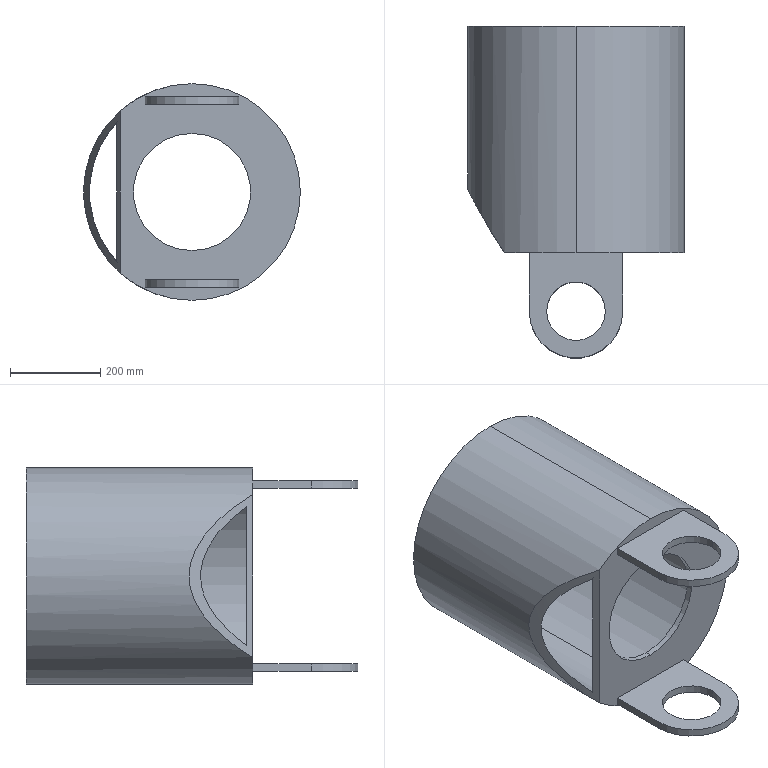Part | SolidWorks | features ICE 3, MoveFace 3, BaseBody 1, Scale 1 | 1 solid | 24 faces | box 481 x 737 x 481 mm | volume 11479821 mm3 | cylinder 13 | plane 11 | commonest cylinder face diameters 130 x4 208 x2 260 x2 455 x2 481 x2 2594 x1
STEP:
#1=CARTESIAN_POINT('',(65.,-174.262,211.9));
#2=VERTEX_POINT('',#1);
#3=CARTESIAN_POINT('',(-65.,-174.262,211.9));
#4=VERTEX_POINT('',#3);
#5=CARTESIAN_POINT('',(0.,-174.262,211.9));
#6=DIRECTION('',(0.,0.,-1.));
#7=DIRECTION('',(1.,0.,0.));
#8=AXIS2_PLACEMENT_3D('',#5,#6,#7);
#9=CIRCLE('',#8,65.);
#10=EDGE_CURVE('',#2,#4,#9,.T.);
#11=ORIENTED_EDGE('',*,*,#10,.F.);
#12=CARTESIAN_POINT('',(65.,-174.262,195.));
#13=VERTEX_POINT('',#12);
#14=CARTESIAN_POINT('',(65.,-174.262,428.84));
#15=DIRECTION('',(0.,0.,-1.));
#16=VECTOR('',#15,1000.);
#17=LINE('',#14,#16);
#18=EDGE_CURVE('',#2,#13,#17,.T.);
#19=ORIENTED_EDGE('',*,*,#18,.T.);
#20=CARTESIAN_POINT('',(-65.,-174.262,195.));
#21=VERTEX_POINT('',#20);
#22=CARTESIAN_POINT('',(0.,-174.262,195.));
#23=DIRECTION('',(0.,0.,-1.));
#24=DIRECTION('',(-1.,0.,0.));
#25=AXIS2_PLACEMENT_3D('',#22,#23,#24);
#26=CIRCLE('',#25,65.);
#27=EDGE_CURVE('',#13,#21,#26,.T.);
#28=ORIENTED_EDGE('',*,*,#27,.T.);
#29=CARTESIAN_POINT('',(-65.,-174.262,428.84));
#30=DIRECTION('',(0.,0.,-1.));
#31=VECTOR('',#30,1000.);
#32=LINE('',#29,#31);
#33=EDGE_CURVE('',#4,#21,#32,.T.);
#34=ORIENTED_EDGE('',*,*,#33,.F.);
#35=EDGE_LOOP('',(#11,#19,#28,#34));
#36=FACE_OUTER_BOUND('',#35,.T.);
#37=CARTESIAN_POINT('',(0.,-174.262,428.84));
#38=DIRECTION('',(0.,0.,-1.));
#39=DIRECTION('',(-1.,0.,0.));
#40=AXIS2_PLACEMENT_3D('',#37,#38,#39);
#41=CYLINDRICAL_SURFACE('',#40,65.);
#42=ADVANCED_FACE('',(#36),#41,.F.);
#43=CARTESIAN_POINT('',(-65.,-174.262,-195.));
#44=VERTEX_POINT('',#43);
#45=CARTESIAN_POINT('',(65.,-174.262,-195.));
#46=VERTEX_POINT('',#45);
#47=CARTESIAN_POINT('',(0.,-174.262,-195.));
#48=DIRECTION('',(0.,0.,1.));
#49=DIRECTION('',(-1.,0.,0.));
#50=AXIS2_PLACEMENT_3D('',#47,#48,#49);
#51=CIRCLE('',#50,65.);
#52=EDGE_CURVE('',#44,#46,#51,.T.);
#53=ORIENTED_EDGE('',*,*,#52,.T.);
#54=CARTESIAN_POINT('',(65.,-174.262,-211.9));
#55=VERTEX_POINT('',#54);
#56=CARTESIAN_POINT('',(65.,-174.262,21.94));
#57=DIRECTION('',(0.,0.,-1.));
#58=VECTOR('',#57,1000.);
#59=LINE('',#56,#58);
#60=EDGE_CURVE('',#46,#55,#59,.T.);
#61=ORIENTED_EDGE('',*,*,#60,.T.);
#62=CARTESIAN_POINT('',(-65.,-174.262,-211.9));
#63=VERTEX_POINT('',#62);
#64=CARTESIAN_POINT('',(0.,-174.262,-211.9));
#65=DIRECTION('',(0.,0.,-1.));
#66=DIRECTION('',(-1.,0.,0.));
#67=AXIS2_PLACEMENT_3D('',#64,#65,#66);
#68=CIRCLE('',#67,65.);
#69=EDGE_CURVE('',#55,#63,#68,.T.);
#70=ORIENTED_EDGE('',*,*,#69,.T.);
#71=CARTESIAN_POINT('',(-65.,-174.262,21.94));
#72=DIRECTION('',(0.,0.,-1.));
#73=VECTOR('',#72,1000.);
#74=LINE('',#71,#73);
#75=EDGE_CURVE('',#44,#63,#74,.T.);
#76=ORIENTED_EDGE('',*,*,#75,.F.);
#77=EDGE_LOOP('',(#53,#61,#70,#76));
#78=FACE_OUTER_BOUND('',#77,.T.);
#79=CARTESIAN_POINT('',(0.,-174.262,21.94));
#80=DIRECTION('',(0.,0.,-1.));
#81=DIRECTION('',(-1.,0.,0.));
#82=AXIS2_PLACEMENT_3D('',#79,#80,#81);
#83=CYLINDRICAL_SURFACE('',#82,65.);
#84=ADVANCED_FACE('',(#78),#83,.F.);
#85=CARTESIAN_POINT('',(0.,458.738,-240.5));
#86=VERTEX_POINT('',#85);
#87=CARTESIAN_POINT('',(0.,458.738,240.5));
#88=VERTEX_POINT('',#87);
#89=CARTESIAN_POINT('',(0.,458.738,0.));
#90=DIRECTION('',(0.,-1.,0.));
#91=DIRECTION('',(0.,0.,-1.));
#92=AXIS2_PLACEMENT_3D('',#89,#90,#91);
#93=CIRCLE('',#92,240.5);
#94=EDGE_CURVE('',#86,#88,#93,.T.);
#95=ORIENTED_EDGE('',*,*,#94,.T.);
#96=CARTESIAN_POINT('',(0.,-44.262,240.5));
#97=VERTEX_POINT('',#96);
#98=CARTESIAN_POINT('',(0.,358.738,240.5));
#99=DIRECTION('',(0.,-1.,0.));
#100=VECTOR('',#99,1000.);
#101=LINE('',#98,#100);
#102=EDGE_CURVE('',#88,#97,#101,.T.);
#103=ORIENTED_EDGE('',*,*,#102,.T.);
#104=CARTESIAN_POINT('',(0.,-44.262,-240.5));
#105=VERTEX_POINT('',#104);
#106=CARTESIAN_POINT('',(0.,-44.262,0.));
#107=DIRECTION('',(0.,1.,0.));
#108=DIRECTION('',(0.,0.,-1.));
#109=AXIS2_PLACEMENT_3D('',#106,#107,#108);
#110=CIRCLE('',#109,240.5);
#111=EDGE_CURVE('',#97,#105,#110,.T.);
#112=ORIENTED_EDGE('',*,*,#111,.T.);
#113=CARTESIAN_POINT('',(0.,358.738,-240.5));
#114=DIRECTION('',(0.,-1.,0.));
#115=VECTOR('',#114,1000.);
#116=LINE('',#113,#115);
#117=EDGE_CURVE('',#86,#105,#116,.T.);
#118=ORIENTED_EDGE('',*,*,#117,.F.);
#119=EDGE_LOOP('',(#95,#103,#112,#118));
#120=FACE_OUTER_BOUND('',#119,.T.);
#121=CARTESIAN_POINT('',(0.,358.738,0.));
#122=DIRECTION('',(0.,-1.,0.));
#123=DIRECTION('',(0.,0.,-1.));
#124=AXIS2_PLACEMENT_3D('',#121,#122,#123);
#125=CYLINDRICAL_SURFACE('',#124,240.5);
#126=ADVANCED_FACE('',(#120),#125,.T.);
#127=CARTESIAN_POINT('',(0.,-31.262,130.));
#128=VERTEX_POINT('',#127);
#129=CARTESIAN_POINT('',(0.,-31.262,-130.));
#130=VERTEX_POINT('',#129);
#131=CARTESIAN_POINT('',(0.,-31.262,0.));
#132=DIRECTION('',(0.,-1.,0.));
#133=DIRECTION('',(0.,0.,-1.));
#134=AXIS2_PLACEMENT_3D('',#131,#132,#133);
#135=CIRCLE('',#134,130.);
#136=EDGE_CURVE('',#128,#130,#135,.T.);
#137=ORIENTED_EDGE('',*,*,#136,.F.);
#138=CARTESIAN_POINT('',(0.,-44.262,130.));
#139=VERTEX_POINT('',#138);
#140=CARTESIAN_POINT('',(0.,358.738,130.));
#141=DIRECTION('',(0.,-1.,0.));
#142=VECTOR('',#141,1000.);
#143=LINE('',#140,#142);
#144=EDGE_CURVE('',#128,#139,#143,.T.);
#145=ORIENTED_EDGE('',*,*,#144,.T.);
#146=CARTESIAN_POINT('',(0.,-44.262,-130.));
#147=VERTEX_POINT('',#146);
#148=CARTESIAN_POINT('',(0.,-44.262,0.));
#149=DIRECTION('',(0.,1.,0.));
#150=DIRECTION('',(0.,0.,-1.));
#151=AXIS2_PLACEMENT_3D('',#148,#149,#150);
#152=CIRCLE('',#151,130.);
#153=EDGE_CURVE('',#147,#139,#152,.T.);
#154=ORIENTED_EDGE('',*,*,#153,.F.);
#155=CARTESIAN_POINT('',(0.,358.738,-130.));
#156=DIRECTION('',(0.,-1.,0.));
#157=VECTOR('',#156,1000.);
#158=LINE('',#155,#157);
#159=EDGE_CURVE('',#130,#147,#158,.T.);
#160=ORIENTED_EDGE('',*,*,#159,.F.);
#161=EDGE_LOOP('',(#137,#145,#154,#160));
#162=FACE_OUTER_BOUND('',#161,.T.);
#163=CARTESIAN_POINT('',(0.,358.738,0.));
#164=DIRECTION('',(0.,-1.,0.));
#165=DIRECTION('',(0.,0.,-1.));
#166=AXIS2_PLACEMENT_3D('',#163,#164,#165);
#167=CYLINDRICAL_SURFACE('',#166,130.);
#168=ADVANCED_FACE('',(#162),#167,.F.);
#169=CARTESIAN_POINT('',(0.,458.738,227.5));
#170=VERTEX_POINT('',#169);
#171=CARTESIAN_POINT('',(0.,458.738,-227.5));
#172=VERTEX_POINT('',#171);
#173=CARTESIAN_POINT('',(0.,458.738,0.));
#174=DIRECTION('',(0.,-1.,0.));
#175=DIRECTION('',(0.,0.,-1.));
#176=AXIS2_PLACEMENT_3D('',#173,#174,#175);
#177=CIRCLE('',#176,227.5);
#178=EDGE_CURVE('',#170,#172,#177,.T.);
#179=ORIENTED_EDGE('',*,*,#178,.F.);
#180=CARTESIAN_POINT('',(0.,-31.262,227.5));
#181=VERTEX_POINT('',#180);
#182=CARTESIAN_POINT('',(0.,358.738,227.5));
#183=DIRECTION('',(0.,-1.,0.));
#184=VECTOR('',#183,1000.);
#185=LINE('',#182,#184);
#186=EDGE_CURVE('',#170,#181,#185,.T.);
#187=ORIENTED_EDGE('',*,*,#186,.T.);
#188=CARTESIAN_POINT('',(-167.294,-31.262,154.171));
#189=VERTEX_POINT('',#188);
#190=CARTESIAN_POINT('',(0.,-31.262,0.));
#191=DIRECTION('',(0.,1.,0.));
#192=DIRECTION('',(0.,0.,-1.));
#193=AXIS2_PLACEMENT_3D('',#190,#191,#192);
#194=CIRCLE('',#193,227.5);
#195=EDGE_CURVE('',#189,#181,#194,.T.);
#196=ORIENTED_EDGE('',*,*,#195,.F.);
#197=CARTESIAN_POINT('',(-167.294,-31.262,-154.171));
#198=VERTEX_POINT('',#197);
#199=CARTESIAN_POINT('',(-167.294,-31.262,154.171));
#200=CARTESIAN_POINT('',(-171.27,-25.129,149.857));
#201=CARTESIAN_POINT('',(-175.109,-19.095,145.358));
#202=CARTESIAN_POINT('',(-182.509,-7.257,135.95));
#203=CARTESIAN_POINT('',(-186.07,-1.453,131.043));
#204=CARTESIAN_POINT('',(-192.904,9.87,120.758));
#205=CARTESIAN_POINT('',(-196.176,15.391,115.382));
#206=CARTESIAN_POINT('',(-202.406,26.071,104.066));
#207=CARTESIAN_POINT('',(-205.365,31.231,98.126));
#208=CARTESIAN_POINT('',(-209.534,38.606,88.677));
#209=CARTESIAN_POINT('',(-210.878,41.004,85.437));
#210=CARTESIAN_POINT('',(-212.82,44.491,80.418));
#211=CARTESIAN_POINT('',(-213.455,45.635,78.718));
#212=CARTESIAN_POINT('',(-214.689,47.867,75.287));
#213=CARTESIAN_POINT('',(-215.289,48.957,73.554));
#214=CARTESIAN_POINT('',(-217.039,52.143,68.294));
#215=CARTESIAN_POINT('',(-218.136,54.155,64.71));
#216=CARTESIAN_POINT('',(-220.181,57.927,57.367));
#217=CARTESIAN_POINT('',(-221.129,59.685,53.609));
#218=CARTESIAN_POINT('',(-222.426,62.104,47.821));
#219=CARTESIAN_POINT('',(-222.837,62.873,45.867));
#220=CARTESIAN_POINT('',(-223.422,63.968,42.896));
#221=CARTESIAN_POINT('',(-223.611,64.322,41.9));
#222=CARTESIAN_POINT('',(-223.975,65.007,39.905));
#223=CARTESIAN_POINT('',(-224.151,65.337,38.905));
#224=CARTESIAN_POINT('',(-224.998,66.932,33.889));
#225=CARTESIAN_POINT('',(-225.573,68.019,29.832));
#226=CARTESIAN_POINT('',(-226.508,69.789,21.62));
#227=CARTESIAN_POINT('',(-226.868,70.473,17.466));
#228=CARTESIAN_POINT('',(-227.236,71.174,11.158));
#229=CARTESIAN_POINT('',(-227.33,71.354,9.043));
#230=CARTESIAN_POINT('',(-227.427,71.538,5.849));
#231=CARTESIAN_POINT('',(-227.452,71.586,4.781));
#232=CARTESIAN_POINT('',(-227.487,71.653,2.639));
#233=CARTESIAN_POINT('',(-227.497,71.672,1.563));
#234=CARTESIAN_POINT('',(-227.518,71.711,-8.121));
#235=CARTESIAN_POINT('',(-227.05,70.816,-16.551));
#236=CARTESIAN_POINT('',(-225.915,68.666,-26.889));
#237=CARTESIAN_POINT('',(-225.66,68.184,-28.947));
#238=CARTESIAN_POINT('',(-225.097,67.119,-33.043));
#239=CARTESIAN_POINT('',(-224.788,66.536,-35.083));
#240=CARTESIAN_POINT('',(-223.782,64.643,-41.165));
#241=CARTESIAN_POINT('',(-223.018,63.208,-45.11));
#242=CARTESIAN_POINT('',(-221.321,60.042,-52.81));
#243=CARTESIAN_POINT('',(-220.389,58.311,-56.565));
#244=CARTESIAN_POINT('',(-218.373,54.59,-63.907));
#245=CARTESIAN_POINT('',(-217.289,52.6,-67.495));
#246=CARTESIAN_POINT('',(-215.557,49.444,-72.765));
#247=CARTESIAN_POINT('',(-214.962,48.363,-74.503));
#248=CARTESIAN_POINT('',(-213.739,46.148,-77.944));
#249=CARTESIAN_POINT('',(-213.109,45.012,-79.649));
#250=CARTESIAN_POINT('',(-211.18,41.544,-84.688));
#251=CARTESIAN_POINT('',(-209.842,39.154,-87.947));
#252=CARTESIAN_POINT('',(-205.683,31.788,-97.461));
#253=CARTESIAN_POINT('',(-202.72,26.615,-103.457));
#254=CARTESIAN_POINT('',(-196.461,15.874,-114.9));
#255=CARTESIAN_POINT('',(-193.163,10.305,-120.347));
#256=CARTESIAN_POINT('',(-187.985,1.717,-128.171));
#257=CARTESIAN_POINT('',(-186.22,-1.185,-130.721));
#258=CARTESIAN_POINT('',(-183.515,-5.592,-134.466));
#259=CARTESIAN_POINT('',(-182.603,-7.071,-135.701));
#260=CARTESIAN_POINT('',(-180.764,-10.041,-138.142));
#261=CARTESIAN_POINT('',(-179.836,-11.533,-139.347));
#262=CARTESIAN_POINT('',(-175.158,-19.019,-145.302));
#263=CARTESIAN_POINT('',(-171.288,-25.102,-149.838));
#264=CARTESIAN_POINT('',(-167.294,-31.262,-154.171));
#265=B_SPLINE_CURVE_WITH_KNOTS('',3,(#199,#200,#201,#202,#203,#204,#205,#206,#207,#208,#209,#210,#211,#212,#213,#214,#215,#216,#217,#218,#219,#220,#221,#222,#223,#224,#225,#226,#227,#228,#229,#230,#231,#232,#233,#234,#235,#236,#237,#238,#239,#240,#241,#242,#243,#244,#245,#246,#247,#248,#249,#250,#251,#252,#253,#254,#255,#256,#257,#258,#259,#260,#261,#262,#263,#264),.UNSPECIFIED.,.F.,.F.,(4,2,2,2,2,2,2,2,2,2,2,2,2,2,2,2,2,2,2,2,2,2,2,2,2,2,2,2,2,2,2,2,4),(0.,0.02512,0.05023,0.07535,0.1005,0.113,0.1193,0.1256,0.1381,0.1507,0.157,0.1601,0.1632,0.1758,0.1884,0.1946,0.1978,0.2009,0.226,0.2323,0.2386,0.2512,0.2637,0.2763,0.2825,0.2888,0.3014,0.3265,0.3516,0.3642,0.3704,0.3767,0.4018),.UNSPECIFIED.);
#266=EDGE_CURVE('',#189,#198,#265,.T.);
#267=ORIENTED_EDGE('',*,*,#266,.T.);
#268=CARTESIAN_POINT('',(0.,-31.262,-227.5));
#269=VERTEX_POINT('',#268);
#270=CARTESIAN_POINT('',(0.,-31.262,0.));
#271=DIRECTION('',(0.,1.,0.));
#272=DIRECTION('',(0.,0.,-1.));
#273=AXIS2_PLACEMENT_3D('',#270,#271,#272);
#274=CIRCLE('',#273,227.5);
#275=EDGE_CURVE('',#269,#198,#274,.T.);
#276=ORIENTED_EDGE('',*,*,#275,.F.);
#277=CARTESIAN_POINT('',(0.,358.738,-227.5));
#278=DIRECTION('',(0.,-1.,0.));
#279=VECTOR('',#278,1000.);
#280=LINE('',#277,#279);
#281=EDGE_CURVE('',#172,#269,#280,.T.);
#282=ORIENTED_EDGE('',*,*,#281,.F.);
#283=EDGE_LOOP('',(#179,#187,#196,#267,#276,#282));
#284=FACE_OUTER_BOUND('',#283,.T.);
#285=CARTESIAN_POINT('',(0.,358.738,0.));
#286=DIRECTION('',(0.,-1.,0.));
#287=DIRECTION('',(0.,0.,-1.));
#288=AXIS2_PLACEMENT_3D('',#285,#286,#287);
#289=CYLINDRICAL_SURFACE('',#288,227.5);
#290=ADVANCED_FACE('',(#284),#289,.F.);
#291=ORIENTED_EDGE('',*,*,#102,.F.);
#292=CARTESIAN_POINT('',(0.,458.738,0.));
#293=DIRECTION('',(0.,-1.,0.));
#294=DIRECTION('',(0.,0.,-1.));
#295=AXIS2_PLACEMENT_3D('',#292,#293,#294);
#296=CIRCLE('',#295,240.5);
#297=EDGE_CURVE('',#88,#86,#296,.T.);
#298=ORIENTED_EDGE('',*,*,#297,.T.);
#299=ORIENTED_EDGE('',*,*,#117,.T.);
#300=CARTESIAN_POINT('',(-158.755,-44.262,-180.658));
#301=VERTEX_POINT('',#300);
#302=CARTESIAN_POINT('',(0.,-44.262,0.));
#303=DIRECTION('',(0.,1.,0.));
#304=DIRECTION('',(0.,0.,-1.));
#305=AXIS2_PLACEMENT_3D('',#302,#303,#304);
#306=CIRCLE('',#305,240.5);
#307=EDGE_CURVE('',#105,#301,#306,.T.);
#308=ORIENTED_EDGE('',*,*,#307,.T.);
#309=CARTESIAN_POINT('',(-158.755,-44.262,180.658));
#310=VERTEX_POINT('',#309);
#311=CARTESIAN_POINT('',(-158.755,-44.262,180.658));
#312=CARTESIAN_POINT('',(-164.07,-36.275,175.987));
#313=CARTESIAN_POINT('',(-169.202,-28.371,171.063));
#314=CARTESIAN_POINT('',(-179.105,-12.764,160.665));
#315=CARTESIAN_POINT('',(-183.876,-5.061,155.192));
#316=CARTESIAN_POINT('',(-193.05,10.09,143.619));
#317=CARTESIAN_POINT('',(-197.454,17.538,137.521));
#318=CARTESIAN_POINT('',(-203.768,28.452,127.804));
#319=CARTESIAN_POINT('',(-205.824,32.046,124.47));
#320=CARTESIAN_POINT('',(-208.831,37.36,119.306));
#321=CARTESIAN_POINT('',(-209.82,39.119,117.558));
#322=CARTESIAN_POINT('',(-211.773,42.608,114.003));
#323=CARTESIAN_POINT('',(-212.735,44.337,112.197));
#324=CARTESIAN_POINT('',(-215.569,49.455,106.71));
#325=CARTESIAN_POINT('',(-217.391,52.781,102.955));
#326=CARTESIAN_POINT('',(-220.888,59.23,95.219));
#327=CARTESIAN_POINT('',(-222.565,62.354,91.239));
#328=CARTESIAN_POINT('',(-224.961,66.861,85.074));
#329=CARTESIAN_POINT('',(-225.74,68.333,82.987));
#330=CARTESIAN_POINT('',(-226.877,70.491,79.802));
#331=CARTESIAN_POINT('',(-227.251,71.202,78.731));
#332=CARTESIAN_POINT('',(-227.988,72.607,76.572));
#333=CARTESIAN_POINT('',(-228.351,73.301,75.482));
#334=CARTESIAN_POINT('',(-230.133,76.713,70.003));
#335=CARTESIAN_POINT('',(-231.453,79.265,65.518));
#336=CARTESIAN_POINT('',(-233.862,83.955,56.314));
#337=CARTESIAN_POINT('',(-234.952,86.094,51.596));
#338=CARTESIAN_POINT('',(-236.876,89.889,41.888));
#339=CARTESIAN_POINT('',(-237.709,91.545,36.9));
#340=CARTESIAN_POINT('',(-238.566,93.255,30.464));
#341=CARTESIAN_POINT('',(-238.729,93.579,29.164));
#342=CARTESIAN_POINT('',(-239.033,94.186,26.559));
#343=CARTESIAN_POINT('',(-239.174,94.469,25.255));
#344=CARTESIAN_POINT('',(-239.566,95.255,21.333));
#345=CARTESIAN_POINT('',(-239.786,95.695,18.71));
#346=CARTESIAN_POINT('',(-240.315,96.757,10.81));
#347=CARTESIAN_POINT('',(-240.496,97.123,5.505));
#348=CARTESIAN_POINT('',(-240.502,97.133,-2.513));
#349=CARTESIAN_POINT('',(-240.459,97.047,-5.198));
#350=CARTESIAN_POINT('',(-240.282,96.692,-10.58));
#351=CARTESIAN_POINT('',(-240.15,96.425,-13.247));
#352=CARTESIAN_POINT('',(-239.624,95.37,-21.179));
#353=CARTESIAN_POINT('',(-239.105,94.329,-26.377));
#354=CARTESIAN_POINT('',(-238.091,92.307,-34.051));
#355=CARTESIAN_POINT('',(-237.714,91.557,-36.588));
#356=CARTESIAN_POINT('',(-237.092,90.322,-40.365));
#357=CARTESIAN_POINT('',(-236.875,89.892,-41.619));
#358=CARTESIAN_POINT('',(-236.422,88.996,-44.117));
#359=CARTESIAN_POINT('',(-236.187,88.531,-45.358));
#360=CARTESIAN_POINT('',(-234.973,86.135,-51.507));
#361=CARTESIAN_POINT('',(-233.876,83.982,-56.258));
#362=CARTESIAN_POINT('',(-231.463,79.286,-65.48));
#363=CARTESIAN_POINT('',(-230.148,76.742,-69.952));
#364=CARTESIAN_POINT('',(-227.32,71.326,-78.656));
#365=CARTESIAN_POINT('',(-225.808,68.454,-82.889));
#366=CARTESIAN_POINT('',(-223.805,64.687,-88.049));
#367=CARTESIAN_POINT('',(-223.399,63.924,-89.076));
#368=CARTESIAN_POINT('',(-222.577,62.386,-91.11));
#369=CARTESIAN_POINT('',(-222.161,61.61,-92.118));
#370=CARTESIAN_POINT('',(-220.902,59.265,-95.116));
#371=CARTESIAN_POINT('',(-220.046,57.677,-97.08));
#372=CARTESIAN_POINT('',(-217.428,52.849,-102.876));
#373=CARTESIAN_POINT('',(-215.617,49.542,-106.612));
#374=CARTESIAN_POINT('',(-211.876,42.784,-113.866));
#375=CARTESIAN_POINT('',(-209.945,39.332,-117.384));
#376=CARTESIAN_POINT('',(-205.97,32.304,-124.226));
#377=CARTESIAN_POINT('',(-203.926,28.728,-127.551));
#378=CARTESIAN_POINT('',(-197.631,17.84,-137.266));
#379=CARTESIAN_POINT('',(-193.217,10.369,-143.398));
#380=CARTESIAN_POINT('',(-187.439,0.8225,-150.7));
#381=CARTESIAN_POINT('',(-186.27,-1.097,-152.142));
#382=CARTESIAN_POINT('',(-183.913,-4.947,-154.983));
#383=CARTESIAN_POINT('',(-182.723,-6.878,-156.384));
#384=CARTESIAN_POINT('',(-179.122,-12.691,-160.528));
#385=CARTESIAN_POINT('',(-176.677,-16.59,-163.213));
#386=CARTESIAN_POINT('',(-169.217,-28.349,-171.05));
#387=CARTESIAN_POINT('',(-164.072,-36.272,-175.985));
#388=CARTESIAN_POINT('',(-158.755,-44.262,-180.658));
#389=B_SPLINE_CURVE_WITH_KNOTS('',3,(#311,#312,#313,#314,#315,#316,#317,#318,#319,#320,#321,#322,#323,#324,#325,#326,#327,#328,#329,#330,#331,#332,#333,#334,#335,#336,#337,#338,#339,#340,#341,#342,#343,#344,#345,#346,#347,#348,#349,#350,#351,#352,#353,#354,#355,#356,#357,#358,#359,#360,#361,#362,#363,#364,#365,#366,#367,#368,#369,#370,#371,#372,#373,#374,#375,#376,#377,#378,#379,#380,#381,#382,#383,#384,#385,#386,#387,#388),.UNSPECIFIED.,.F.,.F.,(4,2,2,2,2,2,2,2,2,2,2,2,2,2,2,2,2,2,2,2,2,2,2,2,2,2,2,2,2,2,2,2,2,2,2,2,2,2,4),(0.,0.03174,0.06347,0.09521,0.1111,0.119,0.1269,0.1428,0.1587,0.1666,0.1706,0.1745,0.1904,0.2063,0.2222,0.2261,0.2301,0.238,0.2539,0.2618,0.2698,0.2856,0.2936,0.2975,0.3015,0.3174,0.3332,0.3491,0.3531,0.357,0.365,0.3808,0.3967,0.4126,0.4443,0.4522,0.4602,0.476,0.5078),.UNSPECIFIED.);
#390=EDGE_CURVE('',#310,#301,#389,.T.);
#391=ORIENTED_EDGE('',*,*,#390,.F.);
#392=CARTESIAN_POINT('',(0.,-44.262,0.));
#393=DIRECTION('',(0.,1.,0.));
#394=DIRECTION('',(0.,0.,-1.));
#395=AXIS2_PLACEMENT_3D('',#392,#393,#394);
#396=CIRCLE('',#395,240.5);
#397=EDGE_CURVE('',#310,#97,#396,.T.);
#398=ORIENTED_EDGE('',*,*,#397,.T.);
#399=EDGE_LOOP('',(#291,#298,#299,#308,#391,#398));
#400=FACE_OUTER_BOUND('',#399,.T.);
#401=CARTESIAN_POINT('',(0.,358.738,0.));
#402=DIRECTION('',(0.,-1.,0.));
#403=DIRECTION('',(0.,0.,-1.));
#404=AXIS2_PLACEMENT_3D('',#401,#402,#403);
#405=CYLINDRICAL_SURFACE('',#404,240.5);
#406=ADVANCED_FACE('',(#400),#405,.T.);
#407=CARTESIAN_POINT('',(-158.755,-44.262,-648.));
#408=DIRECTION('',(0.,0.,1.));
#409=VECTOR('',#408,1000.);
#410=LINE('',#407,#409);
#411=EDGE_CURVE('',#301,#310,#410,.T.);
#412=ORIENTED_EDGE('',*,*,#411,.F.);
#413=ORIENTED_EDGE('',*,*,#307,.F.);
#414=ORIENTED_EDGE('',*,*,#111,.F.);
#415=ORIENTED_EDGE('',*,*,#397,.F.);
#416=EDGE_LOOP('',(#412,#413,#414,#415));
#417=FACE_OUTER_BOUND('',#416,.T.);
#418=CARTESIAN_POINT('',(104.,-44.262,195.));
#419=VERTEX_POINT('',#418);
#420=CARTESIAN_POINT('',(-104.,-44.262,195.));
#421=VERTEX_POINT('',#420);
#422=CARTESIAN_POINT('',(0.,-44.262,195.));
#423=DIRECTION('',(-1.,0.,0.));
#424=VECTOR('',#423,1000.);
#425=LINE('',#422,#424);
#426=EDGE_CURVE('',#419,#421,#425,.T.);
#427=ORIENTED_EDGE('',*,*,#426,.T.);
#428=CARTESIAN_POINT('',(-104.,-44.262,211.9));
#429=VERTEX_POINT('',#428);
#430=CARTESIAN_POINT('',(-104.,-44.262,0.));
#431=DIRECTION('',(0.,0.,1.));
#432=VECTOR('',#431,1000.);
#433=LINE('',#430,#432);
#434=EDGE_CURVE('',#421,#429,#433,.T.);
#435=ORIENTED_EDGE('',*,*,#434,.T.);
#436=CARTESIAN_POINT('',(104.,-44.262,211.9));
#437=VERTEX_POINT('',#436);
#438=CARTESIAN_POINT('',(0.,-44.262,211.9));
#439=DIRECTION('',(1.,0.,0.));
#440=VECTOR('',#439,1000.);
#441=LINE('',#438,#440);
#442=EDGE_CURVE('',#429,#437,#441,.T.);
#443=ORIENTED_EDGE('',*,*,#442,.T.);
#444=CARTESIAN_POINT('',(104.,-44.262,0.));
#445=DIRECTION('',(0.,0.,-1.));
#446=VECTOR('',#445,1000.);
#447=LINE('',#444,#446);
#448=EDGE_CURVE('',#437,#419,#447,.T.);
#449=ORIENTED_EDGE('',*,*,#448,.T.);
#450=EDGE_LOOP('',(#427,#435,#443,#449));
#451=FACE_BOUND('',#450,.T.);
#452=CARTESIAN_POINT('',(-104.,-44.262,-195.));
#453=VERTEX_POINT('',#452);
#454=CARTESIAN_POINT('',(104.,-44.262,-195.));
#455=VERTEX_POINT('',#454);
#456=CARTESIAN_POINT('',(0.,-44.262,-195.));
#457=DIRECTION('',(1.,0.,0.));
#458=VECTOR('',#457,1000.);
#459=LINE('',#456,#458);
#460=EDGE_CURVE('',#453,#455,#459,.T.);
#461=ORIENTED_EDGE('',*,*,#460,.T.);
#462=CARTESIAN_POINT('',(104.,-44.262,-211.9));
#463=VERTEX_POINT('',#462);
#464=CARTESIAN_POINT('',(104.,-44.262,0.));
#465=DIRECTION('',(0.,0.,-1.));
#466=VECTOR('',#465,1000.);
#467=LINE('',#464,#466);
#468=EDGE_CURVE('',#455,#463,#467,.T.);
#469=ORIENTED_EDGE('',*,*,#468,.T.);
#470=CARTESIAN_POINT('',(-104.,-44.262,-211.9));
#471=VERTEX_POINT('',#470);
#472=CARTESIAN_POINT('',(0.,-44.262,-211.9));
#473=DIRECTION('',(-1.,0.,0.));
#474=VECTOR('',#473,1000.);
#475=LINE('',#472,#474);
#476=EDGE_CURVE('',#463,#471,#475,.T.);
#477=ORIENTED_EDGE('',*,*,#476,.T.);
#478=CARTESIAN_POINT('',(-104.,-44.262,0.));
#479=DIRECTION('',(0.,0.,1.));
#480=VECTOR('',#479,1000.);
#481=LINE('',#478,#480);
#482=EDGE_CURVE('',#471,#453,#481,.T.);
#483=ORIENTED_EDGE('',*,*,#482,.T.);
#484=EDGE_LOOP('',(#461,#469,#477,#483));
#485=FACE_BOUND('',#484,.T.);
#486=ORIENTED_EDGE('',*,*,#153,.T.);
#487=CARTESIAN_POINT('',(0.,-44.262,0.));
#488=DIRECTION('',(0.,1.,0.));
#489=DIRECTION('',(0.,0.,-1.));
#490=AXIS2_PLACEMENT_3D('',#487,#488,#489);
#491=CIRCLE('',#490,130.);
#492=EDGE_CURVE('',#139,#147,#491,.T.);
#493=ORIENTED_EDGE('',*,*,#492,.T.);
#494=EDGE_LOOP('',(#486,#493));
#495=FACE_BOUND('',#494,.T.);
#496=CARTESIAN_POINT('',(0.,-44.262,0.));
#497=DIRECTION('',(0.,-1.,0.));
#498=DIRECTION('',(0.,0.,-1.));
#499=AXIS2_PLACEMENT_3D('',#496,#497,#498);
#500=PLANE('',#499);
#501=ADVANCED_FACE('',(#417,#451,#485,#495),#500,.T.);
#502=CARTESIAN_POINT('',(0.,458.738,0.));
#503=DIRECTION('',(0.,-1.,0.));
#504=DIRECTION('',(0.,0.,-1.));
#505=AXIS2_PLACEMENT_3D('',#502,#503,#504);
#506=CIRCLE('',#505,227.5);
#507=EDGE_CURVE('',#172,#170,#506,.T.);
#508=ORIENTED_EDGE('',*,*,#507,.T.);
#509=ORIENTED_EDGE('',*,*,#178,.T.);
#510=EDGE_LOOP('',(#508,#509));
#511=FACE_BOUND('',#510,.T.);
#512=ORIENTED_EDGE('',*,*,#94,.F.);
#513=ORIENTED_EDGE('',*,*,#297,.F.);
#514=EDGE_LOOP('',(#512,#513));
#515=FACE_OUTER_BOUND('',#514,.T.);
#516=CARTESIAN_POINT('',(0.,458.738,0.));
#517=DIRECTION('',(0.,1.,0.));
#518=DIRECTION('',(0.,0.,1.));
#519=AXIS2_PLACEMENT_3D('',#516,#517,#518);
#520=PLANE('',#519);
#521=ADVANCED_FACE('',(#511,#515),#520,.T.);
#522=CARTESIAN_POINT('',(-104.,-174.262,211.9));
#523=VERTEX_POINT('',#522);
#524=CARTESIAN_POINT('',(-104.,-174.262,195.));
#525=VERTEX_POINT('',#524);
#526=CARTESIAN_POINT('',(-104.,-174.262,206.7));
#527=DIRECTION('',(0.,0.,-1.));
#528=VECTOR('',#527,1000.);
#529=LINE('',#526,#528);
#530=EDGE_CURVE('',#523,#525,#529,.T.);
#531=ORIENTED_EDGE('',*,*,#530,.F.);
#532=CARTESIAN_POINT('',(-104.,-174.262,211.9));
#533=DIRECTION('',(0.,-1.,0.));
#534=VECTOR('',#533,1000.);
#535=LINE('',#532,#534);
#536=EDGE_CURVE('',#429,#523,#535,.T.);
#537=ORIENTED_EDGE('',*,*,#536,.F.);
#538=ORIENTED_EDGE('',*,*,#434,.F.);
#539=CARTESIAN_POINT('',(-104.,-174.262,195.));
#540=DIRECTION('',(0.,1.,0.));
#541=VECTOR('',#540,1000.);
#542=LINE('',#539,#541);
#543=EDGE_CURVE('',#525,#421,#542,.T.);
#544=ORIENTED_EDGE('',*,*,#543,.F.);
#545=EDGE_LOOP('',(#531,#537,#538,#544));
#546=FACE_OUTER_BOUND('',#545,.T.);
#547=CARTESIAN_POINT('',(-104.,-174.262,206.7));
#548=DIRECTION('',(1.,0.,0.));
#549=DIRECTION('',(0.,0.,-1.));
#550=AXIS2_PLACEMENT_3D('',#547,#548,#549);
#551=PLANE('',#550);
#552=ADVANCED_FACE('',(#546),#551,.F.);
#553=ORIENTED_EDGE('',*,*,#543,.T.);
#554=ORIENTED_EDGE('',*,*,#426,.F.);
#555=CARTESIAN_POINT('',(104.,-174.262,195.));
#556=VERTEX_POINT('',#555);
#557=CARTESIAN_POINT('',(104.,-174.262,195.));
#558=DIRECTION('',(0.,1.,0.));
#559=VECTOR('',#558,1000.);
#560=LINE('',#557,#559);
#561=EDGE_CURVE('',#556,#419,#560,.T.);
#562=ORIENTED_EDGE('',*,*,#561,.F.);
#563=CARTESIAN_POINT('',(0.,-174.262,195.));
#564=DIRECTION('',(0.,0.,1.));
#565=DIRECTION('',(-1.,0.,0.));
#566=AXIS2_PLACEMENT_3D('',#563,#564,#565);
#567=CIRCLE('',#566,104.);
#568=EDGE_CURVE('',#525,#556,#567,.T.);
#569=ORIENTED_EDGE('',*,*,#568,.F.);
#570=EDGE_LOOP('',(#553,#554,#562,#569));
#571=FACE_OUTER_BOUND('',#570,.T.);
#572=CARTESIAN_POINT('',(0.,-174.262,195.));
#573=DIRECTION('',(0.,0.,-1.));
#574=DIRECTION('',(-1.,0.,0.));
#575=AXIS2_PLACEMENT_3D('',#572,#573,#574);
#576=CIRCLE('',#575,65.);
#577=EDGE_CURVE('',#21,#13,#576,.T.);
#578=ORIENTED_EDGE('',*,*,#577,.F.);
#579=ORIENTED_EDGE('',*,*,#27,.F.);
#580=EDGE_LOOP('',(#578,#579));
#581=FACE_BOUND('',#580,.T.);
#582=CARTESIAN_POINT('',(0.,-174.262,195.));
#583=DIRECTION('',(0.,0.,1.));
#584=DIRECTION('',(1.,0.,0.));
#585=AXIS2_PLACEMENT_3D('',#582,#583,#584);
#586=PLANE('',#585);
#587=ADVANCED_FACE('',(#571,#581),#586,.F.);
#588=ORIENTED_EDGE('',*,*,#448,.F.);
#589=CARTESIAN_POINT('',(104.,-174.262,211.9));
#590=VERTEX_POINT('',#589);
#591=CARTESIAN_POINT('',(104.,-174.262,211.9));
#592=DIRECTION('',(0.,1.,0.));
#593=VECTOR('',#592,1000.);
#594=LINE('',#591,#593);
#595=EDGE_CURVE('',#590,#437,#594,.T.);
#596=ORIENTED_EDGE('',*,*,#595,.F.);
#597=CARTESIAN_POINT('',(104.,-174.262,206.7));
#598=DIRECTION('',(0.,0.,1.));
#599=VECTOR('',#598,1000.);
#600=LINE('',#597,#599);
#601=EDGE_CURVE('',#556,#590,#600,.T.);
#602=ORIENTED_EDGE('',*,*,#601,.F.);
#603=ORIENTED_EDGE('',*,*,#561,.T.);
#604=EDGE_LOOP('',(#588,#596,#602,#603));
#605=FACE_OUTER_BOUND('',#604,.T.);
#606=CARTESIAN_POINT('',(104.,-174.262,206.7));
#607=DIRECTION('',(-1.,0.,0.));
#608=DIRECTION('',(0.,-1.,0.));
#609=AXIS2_PLACEMENT_3D('',#606,#607,#608);
#610=PLANE('',#609);
#611=ADVANCED_FACE('',(#605),#610,.F.);
#612=ORIENTED_EDGE('',*,*,#442,.F.);
#613=ORIENTED_EDGE('',*,*,#536,.T.);
#614=CARTESIAN_POINT('',(0.,-174.262,211.9));
#615=DIRECTION('',(0.,0.,1.));
#616=DIRECTION('',(-1.,0.,0.));
#617=AXIS2_PLACEMENT_3D('',#614,#615,#616);
#618=CIRCLE('',#617,104.);
#619=EDGE_CURVE('',#523,#590,#618,.T.);
#620=ORIENTED_EDGE('',*,*,#619,.T.);
#621=ORIENTED_EDGE('',*,*,#595,.T.);
#622=EDGE_LOOP('',(#612,#613,#620,#621));
#623=FACE_OUTER_BOUND('',#622,.T.);
#624=CARTESIAN_POINT('',(0.,-174.262,211.9));
#625=DIRECTION('',(0.,0.,-1.));
#626=DIRECTION('',(1.,0.,0.));
#627=AXIS2_PLACEMENT_3D('',#624,#625,#626);
#628=CIRCLE('',#627,65.);
#629=EDGE_CURVE('',#4,#2,#628,.T.);
#630=ORIENTED_EDGE('',*,*,#629,.T.);
#631=ORIENTED_EDGE('',*,*,#10,.T.);
#632=EDGE_LOOP('',(#630,#631));
#633=FACE_BOUND('',#632,.T.);
#634=CARTESIAN_POINT('',(0.,-174.262,211.9));
#635=DIRECTION('',(0.,0.,1.));
#636=DIRECTION('',(1.,0.,0.));
#637=AXIS2_PLACEMENT_3D('',#634,#635,#636);
#638=PLANE('',#637);
#639=ADVANCED_FACE('',(#623,#633),#638,.T.);
#640=CARTESIAN_POINT('',(104.,-174.262,-211.9));
#641=VERTEX_POINT('',#640);
#642=CARTESIAN_POINT('',(104.,-174.262,-211.9));
#643=DIRECTION('',(0.,1.,0.));
#644=VECTOR('',#643,1000.);
#645=LINE('',#642,#644);
#646=EDGE_CURVE('',#641,#463,#645,.T.);
#647=ORIENTED_EDGE('',*,*,#646,.T.);
#648=ORIENTED_EDGE('',*,*,#468,.F.);
#649=CARTESIAN_POINT('',(104.,-174.262,-195.));
#650=VERTEX_POINT('',#649);
#651=CARTESIAN_POINT('',(104.,-174.262,-195.));
#652=DIRECTION('',(0.,-1.,0.));
#653=VECTOR('',#652,1000.);
#654=LINE('',#651,#653);
#655=EDGE_CURVE('',#455,#650,#654,.T.);
#656=ORIENTED_EDGE('',*,*,#655,.T.);
#657=CARTESIAN_POINT('',(104.,-174.262,-206.7));
#658=DIRECTION('',(0.,0.,-1.));
#659=VECTOR('',#658,1000.);
#660=LINE('',#657,#659);
#661=EDGE_CURVE('',#650,#641,#660,.T.);
#662=ORIENTED_EDGE('',*,*,#661,.T.);
#663=EDGE_LOOP('',(#647,#648,#656,#662));
#664=FACE_OUTER_BOUND('',#663,.T.);
#665=CARTESIAN_POINT('',(104.,-174.262,-206.7));
#666=DIRECTION('',(1.,0.,0.));
#667=DIRECTION('',(0.,1.,0.));
#668=AXIS2_PLACEMENT_3D('',#665,#666,#667);
#669=PLANE('',#668);
#670=ADVANCED_FACE('',(#664),#669,.T.);
#671=ORIENTED_EDGE('',*,*,#655,.F.);
#672=ORIENTED_EDGE('',*,*,#460,.F.);
#673=CARTESIAN_POINT('',(-104.,-174.262,-195.));
#674=VERTEX_POINT('',#673);
#675=CARTESIAN_POINT('',(-104.,-174.262,-195.));
#676=DIRECTION('',(0.,1.,0.));
#677=VECTOR('',#676,1000.);
#678=LINE('',#675,#677);
#679=EDGE_CURVE('',#674,#453,#678,.T.);
#680=ORIENTED_EDGE('',*,*,#679,.F.);
#681=CARTESIAN_POINT('',(0.,-174.262,-195.));
#682=DIRECTION('',(0.,0.,-1.));
#683=DIRECTION('',(1.,0.,0.));
#684=AXIS2_PLACEMENT_3D('',#681,#682,#683);
#685=CIRCLE('',#684,104.);
#686=EDGE_CURVE('',#650,#674,#685,.T.);
#687=ORIENTED_EDGE('',*,*,#686,.F.);
#688=EDGE_LOOP('',(#671,#672,#680,#687));
#689=FACE_OUTER_BOUND('',#688,.T.);
#690=ORIENTED_EDGE('',*,*,#52,.F.);
#691=CARTESIAN_POINT('',(0.,-174.262,-195.));
#692=DIRECTION('',(0.,0.,1.));
#693=DIRECTION('',(-1.,0.,0.));
#694=AXIS2_PLACEMENT_3D('',#691,#692,#693);
#695=CIRCLE('',#694,65.);
#696=EDGE_CURVE('',#46,#44,#695,.T.);
#697=ORIENTED_EDGE('',*,*,#696,.F.);
#698=EDGE_LOOP('',(#690,#697));
#699=FACE_BOUND('',#698,.T.);
#700=CARTESIAN_POINT('',(0.,-174.262,-195.));
#701=DIRECTION('',(0.,0.,-1.));
#702=DIRECTION('',(-1.,0.,0.));
#703=AXIS2_PLACEMENT_3D('',#700,#701,#702);
#704=PLANE('',#703);
#705=ADVANCED_FACE('',(#689,#699),#704,.F.);
#706=CARTESIAN_POINT('',(-104.,-174.262,-211.9));
#707=VERTEX_POINT('',#706);
#708=CARTESIAN_POINT('',(-104.,-174.262,-211.9));
#709=DIRECTION('',(0.,-1.,0.));
#710=VECTOR('',#709,1000.);
#711=LINE('',#708,#710);
#712=EDGE_CURVE('',#471,#707,#711,.T.);
#713=ORIENTED_EDGE('',*,*,#712,.T.);
#714=CARTESIAN_POINT('',(-104.,-174.262,-206.7));
#715=DIRECTION('',(0.,0.,1.));
#716=VECTOR('',#715,1000.);
#717=LINE('',#714,#716);
#718=EDGE_CURVE('',#707,#674,#717,.T.);
#719=ORIENTED_EDGE('',*,*,#718,.T.);
#720=ORIENTED_EDGE('',*,*,#679,.T.);
#721=ORIENTED_EDGE('',*,*,#482,.F.);
#722=EDGE_LOOP('',(#713,#719,#720,#721));
#723=FACE_OUTER_BOUND('',#722,.T.);
#724=CARTESIAN_POINT('',(-104.,-174.262,-206.7));
#725=DIRECTION('',(-1.,0.,0.));
#726=DIRECTION('',(0.,0.,1.));
#727=AXIS2_PLACEMENT_3D('',#724,#725,#726);
#728=PLANE('',#727);
#729=ADVANCED_FACE('',(#723),#728,.T.);
#730=ORIENTED_EDGE('',*,*,#476,.F.);
#731=ORIENTED_EDGE('',*,*,#646,.F.);
#732=CARTESIAN_POINT('',(0.,-174.262,-211.9));
#733=DIRECTION('',(0.,0.,-1.));
#734=DIRECTION('',(1.,0.,0.));
#735=AXIS2_PLACEMENT_3D('',#732,#733,#734);
#736=CIRCLE('',#735,104.);
#737=EDGE_CURVE('',#641,#707,#736,.T.);
#738=ORIENTED_EDGE('',*,*,#737,.T.);
#739=ORIENTED_EDGE('',*,*,#712,.F.);
#740=EDGE_LOOP('',(#730,#731,#738,#739));
#741=FACE_OUTER_BOUND('',#740,.T.);
#742=CARTESIAN_POINT('',(0.,-174.262,-211.9));
#743=DIRECTION('',(0.,0.,-1.));
#744=DIRECTION('',(-1.,0.,0.));
#745=AXIS2_PLACEMENT_3D('',#742,#743,#744);
#746=CIRCLE('',#745,65.);
#747=EDGE_CURVE('',#63,#55,#746,.T.);
#748=ORIENTED_EDGE('',*,*,#747,.F.);
#749=ORIENTED_EDGE('',*,*,#69,.F.);
#750=EDGE_LOOP('',(#748,#749));
#751=FACE_BOUND('',#750,.T.);
#752=CARTESIAN_POINT('',(0.,-174.262,-211.9));
#753=DIRECTION('',(0.,0.,-1.));
#754=DIRECTION('',(-1.,0.,0.));
#755=AXIS2_PLACEMENT_3D('',#752,#753,#754);
#756=PLANE('',#755);
#757=ADVANCED_FACE('',(#741,#751),#756,.T.);
#758=ORIENTED_EDGE('',*,*,#144,.F.);
#759=CARTESIAN_POINT('',(0.,-31.262,0.));
#760=DIRECTION('',(0.,-1.,0.));
#761=DIRECTION('',(0.,0.,-1.));
#762=AXIS2_PLACEMENT_3D('',#759,#760,#761);
#763=CIRCLE('',#762,130.);
#764=EDGE_CURVE('',#130,#128,#763,.T.);
#765=ORIENTED_EDGE('',*,*,#764,.F.);
#766=ORIENTED_EDGE('',*,*,#159,.T.);
#767=ORIENTED_EDGE('',*,*,#492,.F.);
#768=EDGE_LOOP('',(#758,#765,#766,#767));
#769=FACE_OUTER_BOUND('',#768,.T.);
#770=CARTESIAN_POINT('',(0.,358.738,0.));
#771=DIRECTION('',(0.,-1.,0.));
#772=DIRECTION('',(0.,0.,-1.));
#773=AXIS2_PLACEMENT_3D('',#770,#771,#772);
#774=CYLINDRICAL_SURFACE('',#773,130.);
#775=ADVANCED_FACE('',(#769),#774,.F.);
#776=ORIENTED_EDGE('',*,*,#186,.F.);
#777=ORIENTED_EDGE('',*,*,#507,.F.);
#778=ORIENTED_EDGE('',*,*,#281,.T.);
#779=CARTESIAN_POINT('',(0.,-31.262,0.));
#780=DIRECTION('',(0.,1.,0.));
#781=DIRECTION('',(0.,0.,-1.));
#782=AXIS2_PLACEMENT_3D('',#779,#780,#781);
#783=CIRCLE('',#782,227.5);
#784=EDGE_CURVE('',#181,#269,#783,.T.);
#785=ORIENTED_EDGE('',*,*,#784,.F.);
#786=EDGE_LOOP('',(#776,#777,#778,#785));
#787=FACE_OUTER_BOUND('',#786,.T.);
#788=CARTESIAN_POINT('',(0.,358.738,0.));
#789=DIRECTION('',(0.,-1.,0.));
#790=DIRECTION('',(0.,0.,-1.));
#791=AXIS2_PLACEMENT_3D('',#788,#789,#790);
#792=CYLINDRICAL_SURFACE('',#791,227.5);
#793=ADVANCED_FACE('',(#787),#792,.F.);
#794=ORIENTED_EDGE('',*,*,#619,.F.);
#795=ORIENTED_EDGE('',*,*,#530,.T.);
#796=ORIENTED_EDGE('',*,*,#568,.T.);
#797=ORIENTED_EDGE('',*,*,#601,.T.);
#798=EDGE_LOOP('',(#794,#795,#796,#797));
#799=FACE_OUTER_BOUND('',#798,.T.);
#800=CARTESIAN_POINT('',(0.,-174.262,206.7));
#801=DIRECTION('',(0.,0.,-1.));
#802=DIRECTION('',(-1.,0.,0.));
#803=AXIS2_PLACEMENT_3D('',#800,#801,#802);
#804=CYLINDRICAL_SURFACE('',#803,104.);
#805=ADVANCED_FACE('',(#799),#804,.T.);
#806=ORIENTED_EDGE('',*,*,#737,.F.);
#807=ORIENTED_EDGE('',*,*,#661,.F.);
#808=ORIENTED_EDGE('',*,*,#686,.T.);
#809=ORIENTED_EDGE('',*,*,#718,.F.);
#810=EDGE_LOOP('',(#806,#807,#808,#809));
#811=FACE_OUTER_BOUND('',#810,.T.);
#812=CARTESIAN_POINT('',(0.,-174.262,-206.7));
#813=DIRECTION('',(0.,0.,1.));
#814=DIRECTION('',(1.,0.,0.));
#815=AXIS2_PLACEMENT_3D('',#812,#813,#814);
#816=CYLINDRICAL_SURFACE('',#815,104.);
#817=ADVANCED_FACE('',(#811),#816,.T.);
#818=ORIENTED_EDGE('',*,*,#195,.T.);
#819=ORIENTED_EDGE('',*,*,#784,.T.);
#820=ORIENTED_EDGE('',*,*,#275,.T.);
#821=CARTESIAN_POINT('',(-167.294,-31.262,-648.));
#822=DIRECTION('',(0.,0.,1.));
#823=VECTOR('',#822,1000.);
#824=LINE('',#821,#823);
#825=EDGE_CURVE('',#198,#189,#824,.T.);
#826=ORIENTED_EDGE('',*,*,#825,.T.);
#827=EDGE_LOOP('',(#818,#819,#820,#826));
#828=FACE_OUTER_BOUND('',#827,.T.);
#829=ORIENTED_EDGE('',*,*,#764,.T.);
#830=ORIENTED_EDGE('',*,*,#136,.T.);
#831=EDGE_LOOP('',(#829,#830));
#832=FACE_BOUND('',#831,.T.);
#833=CARTESIAN_POINT('',(0.,-31.262,0.));
#834=DIRECTION('',(0.,-1.,0.));
#835=DIRECTION('',(0.,0.,-1.));
#836=AXIS2_PLACEMENT_3D('',#833,#834,#835);
#837=PLANE('',#836);
#838=ADVANCED_FACE('',(#828,#832),#837,.F.);
#839=ORIENTED_EDGE('',*,*,#60,.F.);
#840=ORIENTED_EDGE('',*,*,#696,.T.);
#841=ORIENTED_EDGE('',*,*,#75,.T.);
#842=ORIENTED_EDGE('',*,*,#747,.T.);
#843=EDGE_LOOP('',(#839,#840,#841,#842));
#844=FACE_OUTER_BOUND('',#843,.T.);
#845=CARTESIAN_POINT('',(0.,-174.262,21.94));
#846=DIRECTION('',(0.,0.,-1.));
#847=DIRECTION('',(-1.,0.,0.));
#848=AXIS2_PLACEMENT_3D('',#845,#846,#847);
#849=CYLINDRICAL_SURFACE('',#848,65.);
#850=ADVANCED_FACE('',(#844),#849,.F.);
#851=ORIENTED_EDGE('',*,*,#18,.F.);
#852=ORIENTED_EDGE('',*,*,#629,.F.);
#853=ORIENTED_EDGE('',*,*,#33,.T.);
#854=ORIENTED_EDGE('',*,*,#577,.T.);
#855=EDGE_LOOP('',(#851,#852,#853,#854));
#856=FACE_OUTER_BOUND('',#855,.T.);
#857=CARTESIAN_POINT('',(0.,-174.262,428.84));
#858=DIRECTION('',(0.,0.,-1.));
#859=DIRECTION('',(-1.,0.,0.));
#860=AXIS2_PLACEMENT_3D('',#857,#858,#859);
#861=CYLINDRICAL_SURFACE('',#860,65.);
#862=ADVANCED_FACE('',(#856),#861,.F.);
#863=ORIENTED_EDGE('',*,*,#411,.T.);
#864=ORIENTED_EDGE('',*,*,#390,.T.);
#865=EDGE_LOOP('',(#863,#864));
#866=FACE_OUTER_BOUND('',#865,.T.);
#867=ORIENTED_EDGE('',*,*,#266,.F.);
#868=ORIENTED_EDGE('',*,*,#825,.F.);
#869=EDGE_LOOP('',(#867,#868));
#870=FACE_BOUND('',#869,.T.);
#871=CARTESIAN_POINT('',(920.899,674.265,-648.));
#872=DIRECTION('',(0.,0.,1.));
#873=DIRECTION('',(1.,0.,0.));
#874=AXIS2_PLACEMENT_3D('',#871,#872,#873);
#875=CYLINDRICAL_SURFACE('',#874,1296.894);
#876=ADVANCED_FACE('',(#866,#870),#875,.T.);
#877=CLOSED_SHELL('',(#42,#84,#126,#168,#290,#406,#501,#521,#552,#587,#611,#639,#670,#705,#729,#757,#775,#793,#805,#817,#838,#850,#862,#876));
#878=MANIFOLD_SOLID_BREP('',#877);
#879=CARTESIAN_POINT('',(0.,0.,0.));
#880=DIRECTION('',(0.,0.,1.));
#881=DIRECTION('',(1.,0.,0.));
#882=AXIS2_PLACEMENT_3D('',#879,#880,#881);
#883=(LENGTH_UNIT()NAMED_UNIT(*)SI_UNIT(.MILLI.,.METRE.));
#884=UNCERTAINTY_MEASURE_WITH_UNIT(LENGTH_MEASURE(0.00001),#883,'','');
#885=(NAMED_UNIT(*)PLANE_ANGLE_UNIT()SI_UNIT($,.RADIAN.));
#886=(NAMED_UNIT(*)SI_UNIT($,.STERADIAN.)SOLID_ANGLE_UNIT());
#887=(GEOMETRIC_REPRESENTATION_CONTEXT(3)GLOBAL_UNCERTAINTY_ASSIGNED_CONTEXT((#884))GLOBAL_UNIT_ASSIGNED_CONTEXT((#883,#885,#886))REPRESENTATION_CONTEXT('',''));
#888=ADVANCED_BREP_SHAPE_REPRESENTATION('',(#878,#882),#887);